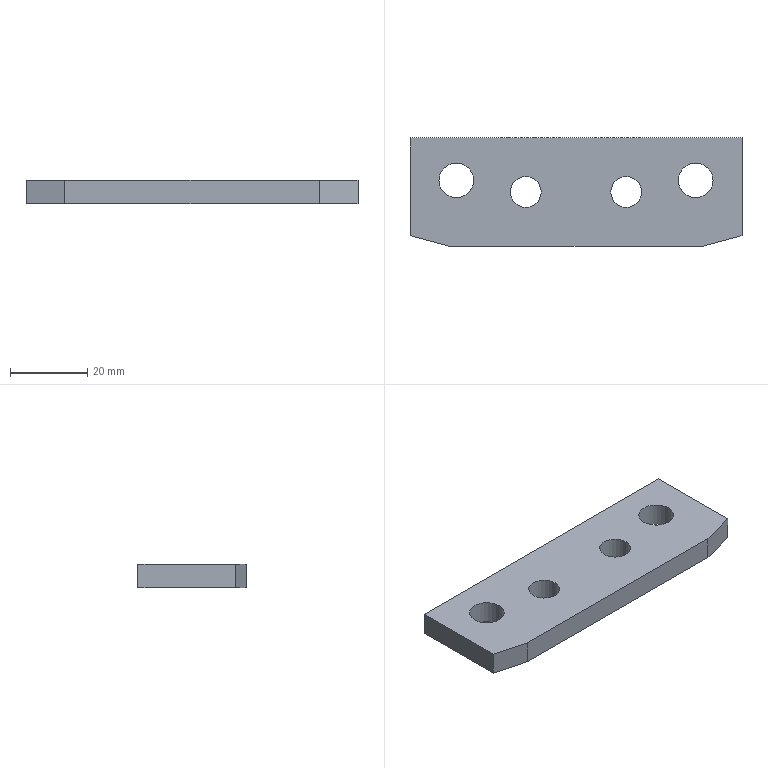Part | STEP file | gslz 2016.10.28-13_id674_x_t | 1 solid | 12 faces | box 86 x 28 x 6 mm | volume 12921 mm3 | plane 8 | cylinder 4 | commonest cylinder face diameters 8 x2 9 x2
STEP:
#1=CARTESIAN_POINT('',(0.,0.,0.));
#2=DIRECTION('',(0.,0.,1.));
#3=DIRECTION('',(1.,0.,0.));
#4=AXIS2_PLACEMENT_3D('',#1,#2,#3);
#5=CARTESIAN_POINT('',(-230.002,281.75,6.));
#6=VERTEX_POINT('',#5);
#7=CARTESIAN_POINT('',(-238.002,281.75,6.));
#8=VERTEX_POINT('',#7);
#9=CARTESIAN_POINT('',(-234.002,281.75,6.));
#10=DIRECTION('',(0.,0.,1.));
#11=DIRECTION('',(-1.,0.,0.));
#12=AXIS2_PLACEMENT_3D('',#9,#10,#11);
#13=CIRCLE('',#12,4.);
#14=CARTESIAN_POINT('',(-234.002,281.75,-73.));
#15=DIRECTION('',(0.,0.,1.));
#16=DIRECTION('',(1.,0.,0.));
#17=AXIS2_PLACEMENT_3D('',#14,#15,#16);
#18=CYLINDRICAL_SURFACE('',#17,4.);
#19=CARTESIAN_POINT('',(-3.142,79.));
#20=DIRECTION('',(1.,0.));
#21=VECTOR('',#20,1.);
#22=LINE('',#19,#21);
#23=(GEOMETRIC_REPRESENTATION_CONTEXT(2)PARAMETRIC_REPRESENTATION_CONTEXT()REPRESENTATION_CONTEXT('',''));
#24=DEFINITIONAL_REPRESENTATION('',(#22),#23);
#25=PCURVE('',#18,#24);
#26=CARTESIAN_POINT('',(-291.002,265.25,6.));
#27=DIRECTION('',(0.,0.,-1.));
#28=DIRECTION('',(-1.,0.,0.));
#29=AXIS2_PLACEMENT_3D('',#26,#27,#28);
#30=PLANE('',#29);
#31=CARTESIAN_POINT('',(-53.,16.5));
#32=CARTESIAN_POINT('',(-53.,9.572));
#33=CARTESIAN_POINT('',(-59.,13.036));
#34=CARTESIAN_POINT('',(-65.,16.5));
#35=CARTESIAN_POINT('',(-59.,19.964));
#36=CARTESIAN_POINT('',(-53.,23.428));
#37=CARTESIAN_POINT('',(-53.,16.5));
#38=(BOUNDED_CURVE()B_SPLINE_CURVE(2,(#31,#32,#33,#34,#35,#36,#37),.UNSPECIFIED.,.T.,.F.)B_SPLINE_CURVE_WITH_KNOTS((1,2,2,2,2,1),(-2.094,0.,2.094,4.189,6.283,8.378),.UNSPECIFIED.)CURVE()GEOMETRIC_REPRESENTATION_ITEM()RATIONAL_B_SPLINE_CURVE((1.,0.5,1.,0.5,1.,0.5,1.))REPRESENTATION_ITEM(''));
#39=(GEOMETRIC_REPRESENTATION_CONTEXT(2)PARAMETRIC_REPRESENTATION_CONTEXT()REPRESENTATION_CONTEXT('',''));
#40=DEFINITIONAL_REPRESENTATION('',(#38),#39);
#41=PCURVE('',#30,#40);
#42=SURFACE_CURVE('',#13,(#25,#41),.PCURVE_S1.);
#43=EDGE_CURVE('',#6,#8,#42,.T.);
#44=ORIENTED_EDGE('',*,*,#43,.F.);
#45=CARTESIAN_POINT('',(-230.002,281.75,0.));
#46=VERTEX_POINT('',#45);
#47=CARTESIAN_POINT('',(-230.002,281.75,0.));
#48=CARTESIAN_POINT('',(-230.002,281.75,6.));
#49=B_SPLINE_CURVE_WITH_KNOTS('',1,(#47,#48),.UNSPECIFIED.,.F.,.F.,(2,2),(73.,79.),.PIECEWISE_BEZIER_KNOTS.);
#50=CARTESIAN_POINT('',(0.,0.));
#51=DIRECTION('',(0.,1.));
#52=VECTOR('',#51,1.);
#53=LINE('',#50,#52);
#54=(GEOMETRIC_REPRESENTATION_CONTEXT(2)PARAMETRIC_REPRESENTATION_CONTEXT()REPRESENTATION_CONTEXT('',''));
#55=DEFINITIONAL_REPRESENTATION('',(#53),#54);
#56=PCURVE('',#18,#55);
#57=CARTESIAN_POINT('',(6.283,0.));
#58=DIRECTION('',(0.,1.));
#59=VECTOR('',#58,1.);
#60=LINE('',#57,#59);
#61=(GEOMETRIC_REPRESENTATION_CONTEXT(2)PARAMETRIC_REPRESENTATION_CONTEXT()REPRESENTATION_CONTEXT('',''));
#62=DEFINITIONAL_REPRESENTATION('',(#60),#61);
#63=PCURVE('',#18,#62);
#64=SEAM_CURVE('',#49,(#56,#63),.PCURVE_S1.);
#65=EDGE_CURVE('',#46,#6,#64,.T.);
#66=ORIENTED_EDGE('',*,*,#65,.F.);
#67=CARTESIAN_POINT('',(-234.002,281.75,0.));
#68=DIRECTION('',(0.,0.,-1.));
#69=DIRECTION('',(1.,0.,0.));
#70=AXIS2_PLACEMENT_3D('',#67,#68,#69);
#71=CIRCLE('',#70,4.);
#72=CARTESIAN_POINT('',(6.283,73.));
#73=DIRECTION('',(-1.,0.));
#74=VECTOR('',#73,1.);
#75=LINE('',#72,#74);
#76=(GEOMETRIC_REPRESENTATION_CONTEXT(2)PARAMETRIC_REPRESENTATION_CONTEXT()REPRESENTATION_CONTEXT('',''));
#77=DEFINITIONAL_REPRESENTATION('',(#75),#76);
#78=PCURVE('',#18,#77);
#79=CARTESIAN_POINT('',(-331.002,295.75,0.));
#80=DIRECTION('',(0.,0.,1.));
#81=DIRECTION('',(1.,0.,0.));
#82=AXIS2_PLACEMENT_3D('',#79,#80,#81);
#83=PLANE('',#82);
#84=CARTESIAN_POINT('',(101.,-14.));
#85=CARTESIAN_POINT('',(101.,-20.928));
#86=CARTESIAN_POINT('',(95.,-17.464));
#87=CARTESIAN_POINT('',(89.,-14.));
#88=CARTESIAN_POINT('',(95.,-10.536));
#89=CARTESIAN_POINT('',(101.,-7.072));
#90=CARTESIAN_POINT('',(101.,-14.));
#91=(BOUNDED_CURVE()B_SPLINE_CURVE(2,(#84,#85,#86,#87,#88,#89,#90),.UNSPECIFIED.,.T.,.F.)B_SPLINE_CURVE_WITH_KNOTS((1,2,2,2,2,1),(-2.094,0.,2.094,4.189,6.283,8.378),.UNSPECIFIED.)CURVE()GEOMETRIC_REPRESENTATION_ITEM()RATIONAL_B_SPLINE_CURVE((1.,0.5,1.,0.5,1.,0.5,1.))REPRESENTATION_ITEM(''));
#92=(GEOMETRIC_REPRESENTATION_CONTEXT(2)PARAMETRIC_REPRESENTATION_CONTEXT()REPRESENTATION_CONTEXT('',''));
#93=DEFINITIONAL_REPRESENTATION('',(#91),#92);
#94=PCURVE('',#83,#93);
#95=SURFACE_CURVE('',#71,(#78,#94),.PCURVE_S1.);
#96=EDGE_CURVE('',#46,#46,#95,.T.);
#97=ORIENTED_EDGE('',*,*,#96,.F.);
#98=ORIENTED_EDGE('',*,*,#65,.T.);
#99=CARTESIAN_POINT('',(-234.002,281.75,6.));
#100=DIRECTION('',(0.,0.,1.));
#101=DIRECTION('',(-1.,0.,0.));
#102=AXIS2_PLACEMENT_3D('',#99,#100,#101);
#103=CIRCLE('',#102,4.);
#104=CARTESIAN_POINT('',(3.142,79.));
#105=DIRECTION('',(1.,0.));
#106=VECTOR('',#105,1.);
#107=LINE('',#104,#106);
#108=(GEOMETRIC_REPRESENTATION_CONTEXT(2)PARAMETRIC_REPRESENTATION_CONTEXT()REPRESENTATION_CONTEXT('',''));
#109=DEFINITIONAL_REPRESENTATION('',(#107),#108);
#110=PCURVE('',#18,#109);
#111=CARTESIAN_POINT('',(-53.,16.5));
#112=CARTESIAN_POINT('',(-53.,9.572));
#113=CARTESIAN_POINT('',(-59.,13.036));
#114=CARTESIAN_POINT('',(-65.,16.5));
#115=CARTESIAN_POINT('',(-59.,19.964));
#116=CARTESIAN_POINT('',(-53.,23.428));
#117=CARTESIAN_POINT('',(-53.,16.5));
#118=(BOUNDED_CURVE()B_SPLINE_CURVE(2,(#111,#112,#113,#114,#115,#116,#117),.UNSPECIFIED.,.T.,.F.)B_SPLINE_CURVE_WITH_KNOTS((1,2,2,2,2,1),(-2.094,0.,2.094,4.189,6.283,8.378),.UNSPECIFIED.)CURVE()GEOMETRIC_REPRESENTATION_ITEM()RATIONAL_B_SPLINE_CURVE((1.,0.5,1.,0.5,1.,0.5,1.))REPRESENTATION_ITEM(''));
#119=(GEOMETRIC_REPRESENTATION_CONTEXT(2)PARAMETRIC_REPRESENTATION_CONTEXT()REPRESENTATION_CONTEXT('',''));
#120=DEFINITIONAL_REPRESENTATION('',(#118),#119);
#121=PCURVE('',#30,#120);
#122=SURFACE_CURVE('',#103,(#110,#121),.PCURVE_S1.);
#123=EDGE_CURVE('',#8,#6,#122,.T.);
#124=ORIENTED_EDGE('',*,*,#123,.F.);
#125=EDGE_LOOP('',(#44,#66,#97,#98,#124));
#126=FACE_BOUND('',#125,.F.);
#127=ADVANCED_FACE('',(#126),#18,.F.);
#128=CARTESIAN_POINT('',(-212.002,281.75,6.));
#129=VERTEX_POINT('',#128);
#130=CARTESIAN_POINT('',(-204.002,281.75,6.));
#131=VERTEX_POINT('',#130);
#132=CARTESIAN_POINT('',(-208.002,281.75,6.));
#133=DIRECTION('',(0.,0.,-1.));
#134=DIRECTION('',(-1.,0.,0.));
#135=AXIS2_PLACEMENT_3D('',#132,#133,#134);
#136=CIRCLE('',#135,4.);
#137=CARTESIAN_POINT('',(-208.002,281.75,-73.));
#138=DIRECTION('',(0.,0.,1.));
#139=DIRECTION('',(1.,0.,0.));
#140=AXIS2_PLACEMENT_3D('',#137,#138,#139);
#141=CYLINDRICAL_SURFACE('',#140,4.);
#142=CARTESIAN_POINT('',(3.142,79.));
#143=DIRECTION('',(-1.,0.));
#144=VECTOR('',#143,1.);
#145=LINE('',#142,#144);
#146=(GEOMETRIC_REPRESENTATION_CONTEXT(2)PARAMETRIC_REPRESENTATION_CONTEXT()REPRESENTATION_CONTEXT('',''));
#147=DEFINITIONAL_REPRESENTATION('',(#145),#146);
#148=PCURVE('',#141,#147);
#149=CARTESIAN_POINT('',(-83.,16.5));
#150=DIRECTION('',(1.,0.));
#151=AXIS2_PLACEMENT_2D('',#149,#150);
#152=CIRCLE('',#151,4.);
#153=(GEOMETRIC_REPRESENTATION_CONTEXT(2)PARAMETRIC_REPRESENTATION_CONTEXT()REPRESENTATION_CONTEXT('',''));
#154=DEFINITIONAL_REPRESENTATION('',(#152),#153);
#155=PCURVE('',#30,#154);
#156=SURFACE_CURVE('',#136,(#148,#155),.PCURVE_S1.);
#157=EDGE_CURVE('',#129,#131,#156,.T.);
#158=ORIENTED_EDGE('',*,*,#157,.T.);
#159=CARTESIAN_POINT('',(-204.002,281.75,0.));
#160=VERTEX_POINT('',#159);
#161=CARTESIAN_POINT('',(-204.002,281.75,0.));
#162=CARTESIAN_POINT('',(-204.002,281.75,6.));
#163=B_SPLINE_CURVE_WITH_KNOTS('',1,(#161,#162),.UNSPECIFIED.,.F.,.F.,(2,2),(73.,79.),.PIECEWISE_BEZIER_KNOTS.);
#164=CARTESIAN_POINT('',(0.,0.));
#165=DIRECTION('',(0.,1.));
#166=VECTOR('',#165,1.);
#167=LINE('',#164,#166);
#168=(GEOMETRIC_REPRESENTATION_CONTEXT(2)PARAMETRIC_REPRESENTATION_CONTEXT()REPRESENTATION_CONTEXT('',''));
#169=DEFINITIONAL_REPRESENTATION('',(#167),#168);
#170=PCURVE('',#141,#169);
#171=CARTESIAN_POINT('',(6.283,0.));
#172=DIRECTION('',(0.,1.));
#173=VECTOR('',#172,1.);
#174=LINE('',#171,#173);
#175=(GEOMETRIC_REPRESENTATION_CONTEXT(2)PARAMETRIC_REPRESENTATION_CONTEXT()REPRESENTATION_CONTEXT('',''));
#176=DEFINITIONAL_REPRESENTATION('',(#174),#175);
#177=PCURVE('',#141,#176);
#178=SEAM_CURVE('',#163,(#170,#177),.PCURVE_S1.);
#179=EDGE_CURVE('',#160,#131,#178,.T.);
#180=ORIENTED_EDGE('',*,*,#179,.F.);
#181=CARTESIAN_POINT('',(-208.002,281.75,0.));
#182=DIRECTION('',(0.,0.,1.));
#183=DIRECTION('',(1.,0.,0.));
#184=AXIS2_PLACEMENT_3D('',#181,#182,#183);
#185=CIRCLE('',#184,4.);
#186=CARTESIAN_POINT('',(0.,73.));
#187=DIRECTION('',(1.,0.));
#188=VECTOR('',#187,1.);
#189=LINE('',#186,#188);
#190=(GEOMETRIC_REPRESENTATION_CONTEXT(2)PARAMETRIC_REPRESENTATION_CONTEXT()REPRESENTATION_CONTEXT('',''));
#191=DEFINITIONAL_REPRESENTATION('',(#189),#190);
#192=PCURVE('',#141,#191);
#193=CARTESIAN_POINT('',(123.,-14.));
#194=DIRECTION('',(1.,0.));
#195=AXIS2_PLACEMENT_2D('',#193,#194);
#196=CIRCLE('',#195,4.);
#197=(GEOMETRIC_REPRESENTATION_CONTEXT(2)PARAMETRIC_REPRESENTATION_CONTEXT()REPRESENTATION_CONTEXT('',''));
#198=DEFINITIONAL_REPRESENTATION('',(#196),#197);
#199=PCURVE('',#83,#198);
#200=SURFACE_CURVE('',#185,(#192,#199),.PCURVE_S1.);
#201=EDGE_CURVE('',#160,#160,#200,.T.);
#202=ORIENTED_EDGE('',*,*,#201,.T.);
#203=ORIENTED_EDGE('',*,*,#179,.T.);
#204=CARTESIAN_POINT('',(-208.002,281.75,6.));
#205=DIRECTION('',(0.,0.,-1.));
#206=DIRECTION('',(-1.,0.,0.));
#207=AXIS2_PLACEMENT_3D('',#204,#205,#206);
#208=CIRCLE('',#207,4.);
#209=CARTESIAN_POINT('',(9.425,79.));
#210=DIRECTION('',(-1.,0.));
#211=VECTOR('',#210,1.);
#212=LINE('',#209,#211);
#213=(GEOMETRIC_REPRESENTATION_CONTEXT(2)PARAMETRIC_REPRESENTATION_CONTEXT()REPRESENTATION_CONTEXT('',''));
#214=DEFINITIONAL_REPRESENTATION('',(#212),#213);
#215=PCURVE('',#141,#214);
#216=CARTESIAN_POINT('',(-83.,16.5));
#217=DIRECTION('',(1.,0.));
#218=AXIS2_PLACEMENT_2D('',#216,#217);
#219=CIRCLE('',#218,4.);
#220=(GEOMETRIC_REPRESENTATION_CONTEXT(2)PARAMETRIC_REPRESENTATION_CONTEXT()REPRESENTATION_CONTEXT('',''));
#221=DEFINITIONAL_REPRESENTATION('',(#219),#220);
#222=PCURVE('',#30,#221);
#223=SURFACE_CURVE('',#208,(#215,#222),.PCURVE_S1.);
#224=EDGE_CURVE('',#131,#129,#223,.T.);
#225=ORIENTED_EDGE('',*,*,#224,.T.);
#226=EDGE_LOOP('',(#158,#180,#202,#203,#225));
#227=FACE_BOUND('',#226,.F.);
#228=ADVANCED_FACE('',(#227),#141,.F.);
#229=CARTESIAN_POINT('',(-256.502,284.75,6.));
#230=VERTEX_POINT('',#229);
#231=CARTESIAN_POINT('',(-252.002,284.75,6.));
#232=DIRECTION('',(0.,0.,-1.));
#233=DIRECTION('',(-1.,0.,0.));
#234=AXIS2_PLACEMENT_3D('',#231,#232,#233);
#235=CIRCLE('',#234,4.5);
#236=CARTESIAN_POINT('',(-252.002,284.75,47.));
#237=DIRECTION('',(0.,0.,-1.));
#238=DIRECTION('',(-1.,0.,0.));
#239=AXIS2_PLACEMENT_3D('',#236,#237,#238);
#240=CYLINDRICAL_SURFACE('',#239,4.5);
#241=CARTESIAN_POINT('',(0.,41.));
#242=DIRECTION('',(1.,0.));
#243=VECTOR('',#242,1.);
#244=LINE('',#241,#243);
#245=(GEOMETRIC_REPRESENTATION_CONTEXT(2)PARAMETRIC_REPRESENTATION_CONTEXT()REPRESENTATION_CONTEXT('',''));
#246=DEFINITIONAL_REPRESENTATION('',(#244),#245);
#247=PCURVE('',#240,#246);
#248=CARTESIAN_POINT('',(-39.,19.5));
#249=DIRECTION('',(1.,0.));
#250=AXIS2_PLACEMENT_2D('',#248,#249);
#251=CIRCLE('',#250,4.5);
#252=(GEOMETRIC_REPRESENTATION_CONTEXT(2)PARAMETRIC_REPRESENTATION_CONTEXT()REPRESENTATION_CONTEXT('',''));
#253=DEFINITIONAL_REPRESENTATION('',(#251),#252);
#254=PCURVE('',#30,#253);
#255=SURFACE_CURVE('',#235,(#247,#254),.PCURVE_S1.);
#256=EDGE_CURVE('',#230,#230,#255,.T.);
#257=ORIENTED_EDGE('',*,*,#256,.T.);
#258=CARTESIAN_POINT('',(-256.502,284.75,0.));
#259=VERTEX_POINT('',#258);
#260=CARTESIAN_POINT('',(-256.502,284.75,6.));
#261=CARTESIAN_POINT('',(-256.502,284.75,0.));
#262=B_SPLINE_CURVE_WITH_KNOTS('',1,(#260,#261),.UNSPECIFIED.,.F.,.F.,(2,2),(41.,47.),.PIECEWISE_BEZIER_KNOTS.);
#263=CARTESIAN_POINT('',(6.283,0.));
#264=DIRECTION('',(0.,1.));
#265=VECTOR('',#264,1.);
#266=LINE('',#263,#265);
#267=(GEOMETRIC_REPRESENTATION_CONTEXT(2)PARAMETRIC_REPRESENTATION_CONTEXT()REPRESENTATION_CONTEXT('',''));
#268=DEFINITIONAL_REPRESENTATION('',(#266),#267);
#269=PCURVE('',#240,#268);
#270=CARTESIAN_POINT('',(0.,0.));
#271=DIRECTION('',(0.,1.));
#272=VECTOR('',#271,1.);
#273=LINE('',#270,#272);
#274=(GEOMETRIC_REPRESENTATION_CONTEXT(2)PARAMETRIC_REPRESENTATION_CONTEXT()REPRESENTATION_CONTEXT('',''));
#275=DEFINITIONAL_REPRESENTATION('',(#273),#274);
#276=PCURVE('',#240,#275);
#277=SEAM_CURVE('',#262,(#269,#276),.PCURVE_S1.);
#278=EDGE_CURVE('',#230,#259,#277,.T.);
#279=ORIENTED_EDGE('',*,*,#278,.T.);
#280=CARTESIAN_POINT('',(-247.502,284.75,0.));
#281=VERTEX_POINT('',#280);
#282=CARTESIAN_POINT('',(-252.002,284.75,0.));
#283=DIRECTION('',(0.,0.,1.));
#284=DIRECTION('',(1.,0.,0.));
#285=AXIS2_PLACEMENT_3D('',#282,#283,#284);
#286=CIRCLE('',#285,4.5);
#287=CARTESIAN_POINT('',(9.425,47.));
#288=DIRECTION('',(-1.,0.));
#289=VECTOR('',#288,1.);
#290=LINE('',#287,#289);
#291=(GEOMETRIC_REPRESENTATION_CONTEXT(2)PARAMETRIC_REPRESENTATION_CONTEXT()REPRESENTATION_CONTEXT('',''));
#292=DEFINITIONAL_REPRESENTATION('',(#290),#291);
#293=PCURVE('',#240,#292);
#294=CARTESIAN_POINT('',(79.,-11.));
#295=DIRECTION('',(1.,0.));
#296=AXIS2_PLACEMENT_2D('',#294,#295);
#297=CIRCLE('',#296,4.5);
#298=(GEOMETRIC_REPRESENTATION_CONTEXT(2)PARAMETRIC_REPRESENTATION_CONTEXT()REPRESENTATION_CONTEXT('',''));
#299=DEFINITIONAL_REPRESENTATION('',(#297),#298);
#300=PCURVE('',#83,#299);
#301=SURFACE_CURVE('',#286,(#293,#300),.PCURVE_S1.);
#302=EDGE_CURVE('',#259,#281,#301,.T.);
#303=ORIENTED_EDGE('',*,*,#302,.T.);
#304=CARTESIAN_POINT('',(-252.002,284.75,0.));
#305=DIRECTION('',(0.,0.,1.));
#306=DIRECTION('',(1.,0.,0.));
#307=AXIS2_PLACEMENT_3D('',#304,#305,#306);
#308=CIRCLE('',#307,4.5);
#309=CARTESIAN_POINT('',(3.142,47.));
#310=DIRECTION('',(-1.,0.));
#311=VECTOR('',#310,1.);
#312=LINE('',#309,#311);
#313=(GEOMETRIC_REPRESENTATION_CONTEXT(2)PARAMETRIC_REPRESENTATION_CONTEXT()REPRESENTATION_CONTEXT('',''));
#314=DEFINITIONAL_REPRESENTATION('',(#312),#313);
#315=PCURVE('',#240,#314);
#316=CARTESIAN_POINT('',(79.,-11.));
#317=DIRECTION('',(1.,0.));
#318=AXIS2_PLACEMENT_2D('',#316,#317);
#319=CIRCLE('',#318,4.5);
#320=(GEOMETRIC_REPRESENTATION_CONTEXT(2)PARAMETRIC_REPRESENTATION_CONTEXT()REPRESENTATION_CONTEXT('',''));
#321=DEFINITIONAL_REPRESENTATION('',(#319),#320);
#322=PCURVE('',#83,#321);
#323=SURFACE_CURVE('',#308,(#315,#322),.PCURVE_S1.);
#324=EDGE_CURVE('',#281,#259,#323,.T.);
#325=ORIENTED_EDGE('',*,*,#324,.T.);
#326=ORIENTED_EDGE('',*,*,#278,.F.);
#327=EDGE_LOOP('',(#257,#279,#303,#325,#326));
#328=FACE_BOUND('',#327,.F.);
#329=ADVANCED_FACE('',(#328),#240,.F.);
#330=CARTESIAN_POINT('',(-188.001,267.75,0.));
#331=VERTEX_POINT('',#330);
#332=CARTESIAN_POINT('',(-188.001,267.75,6.));
#333=VERTEX_POINT('',#332);
#334=CARTESIAN_POINT('',(-188.001,267.75,8.));
#335=DIRECTION('',(0.,0.,1.));
#336=VECTOR('',#335,1.);
#337=LINE('',#334,#336);
#338=CARTESIAN_POINT('',(-321.,267.75,8.));
#339=DIRECTION('',(0.,1.,0.));
#340=DIRECTION('',(0.,0.,1.));
#341=AXIS2_PLACEMENT_3D('',#338,#339,#340);
#342=PLANE('',#341);
#343=CARTESIAN_POINT('',(0.,132.999));
#344=DIRECTION('',(1.,0.));
#345=VECTOR('',#344,1.);
#346=LINE('',#343,#345);
#347=(GEOMETRIC_REPRESENTATION_CONTEXT(2)PARAMETRIC_REPRESENTATION_CONTEXT()REPRESENTATION_CONTEXT('',''));
#348=DEFINITIONAL_REPRESENTATION('',(#346),#347);
#349=PCURVE('',#342,#348);
#350=CARTESIAN_POINT('',(-188.001,267.75,8.));
#351=DIRECTION('',(-0.2588,0.9659,0.));
#352=DIRECTION('',(-0.9659,-0.2588,0.));
#353=AXIS2_PLACEMENT_3D('',#350,#351,#352);
#354=PLANE('',#353);
#355=CARTESIAN_POINT('',(0.,0.));
#356=DIRECTION('',(0.,1.));
#357=VECTOR('',#356,1.);
#358=LINE('',#355,#357);
#359=(GEOMETRIC_REPRESENTATION_CONTEXT(2)PARAMETRIC_REPRESENTATION_CONTEXT()REPRESENTATION_CONTEXT('',''));
#360=DEFINITIONAL_REPRESENTATION('',(#358),#359);
#361=PCURVE('',#354,#360);
#362=SURFACE_CURVE('',#337,(#349,#361),.PCURVE_S1.);
#363=EDGE_CURVE('',#331,#333,#362,.T.);
#364=ORIENTED_EDGE('',*,*,#363,.T.);
#365=CARTESIAN_POINT('',(-254.,267.75,6.));
#366=VERTEX_POINT('',#365);
#367=CARTESIAN_POINT('',(-321.,267.75,6.));
#368=DIRECTION('',(-1.,0.,0.));
#369=VECTOR('',#368,1.);
#370=LINE('',#367,#369);
#371=CARTESIAN_POINT('',(-2.,0.));
#372=DIRECTION('',(0.,-1.));
#373=VECTOR('',#372,1.);
#374=LINE('',#371,#373);
#375=(GEOMETRIC_REPRESENTATION_CONTEXT(2)PARAMETRIC_REPRESENTATION_CONTEXT()REPRESENTATION_CONTEXT('',''));
#376=DEFINITIONAL_REPRESENTATION('',(#374),#375);
#377=PCURVE('',#342,#376);
#378=CARTESIAN_POINT('',(29.998,2.5));
#379=DIRECTION('',(1.,0.));
#380=VECTOR('',#379,1.);
#381=LINE('',#378,#380);
#382=(GEOMETRIC_REPRESENTATION_CONTEXT(2)PARAMETRIC_REPRESENTATION_CONTEXT()REPRESENTATION_CONTEXT('',''));
#383=DEFINITIONAL_REPRESENTATION('',(#381),#382);
#384=PCURVE('',#30,#383);
#385=SURFACE_CURVE('',#370,(#377,#384),.PCURVE_S1.);
#386=EDGE_CURVE('',#333,#366,#385,.T.);
#387=ORIENTED_EDGE('',*,*,#386,.T.);
#388=CARTESIAN_POINT('',(-254.,267.75,0.));
#389=VERTEX_POINT('',#388);
#390=CARTESIAN_POINT('',(-254.,267.75,8.));
#391=DIRECTION('',(0.,0.,1.));
#392=VECTOR('',#391,1.);
#393=LINE('',#390,#392);
#394=CARTESIAN_POINT('',(0.,67.));
#395=DIRECTION('',(1.,0.));
#396=VECTOR('',#395,1.);
#397=LINE('',#394,#396);
#398=(GEOMETRIC_REPRESENTATION_CONTEXT(2)PARAMETRIC_REPRESENTATION_CONTEXT()REPRESENTATION_CONTEXT('',''));
#399=DEFINITIONAL_REPRESENTATION('',(#397),#398);
#400=PCURVE('',#342,#399);
#401=CARTESIAN_POINT('',(-264.002,270.43,8.));
#402=DIRECTION('',(0.2588,0.9659,0.));
#403=DIRECTION('',(-0.9659,0.2588,0.));
#404=AXIS2_PLACEMENT_3D('',#401,#402,#403);
#405=PLANE('',#404);
#406=CARTESIAN_POINT('',(-10.355,0.));
#407=DIRECTION('',(0.,1.));
#408=VECTOR('',#407,1.);
#409=LINE('',#406,#408);
#410=(GEOMETRIC_REPRESENTATION_CONTEXT(2)PARAMETRIC_REPRESENTATION_CONTEXT()REPRESENTATION_CONTEXT('',''));
#411=DEFINITIONAL_REPRESENTATION('',(#409),#410);
#412=PCURVE('',#405,#411);
#413=SURFACE_CURVE('',#393,(#400,#412),.PCURVE_S1.);
#414=EDGE_CURVE('',#389,#366,#413,.T.);
#415=ORIENTED_EDGE('',*,*,#414,.F.);
#416=CARTESIAN_POINT('',(-321.,267.75,0.));
#417=DIRECTION('',(1.,0.,0.));
#418=VECTOR('',#417,1.);
#419=LINE('',#416,#418);
#420=CARTESIAN_POINT('',(-8.,0.));
#421=DIRECTION('',(0.,1.));
#422=VECTOR('',#421,1.);
#423=LINE('',#420,#422);
#424=(GEOMETRIC_REPRESENTATION_CONTEXT(2)PARAMETRIC_REPRESENTATION_CONTEXT()REPRESENTATION_CONTEXT('',''));
#425=DEFINITIONAL_REPRESENTATION('',(#423),#424);
#426=PCURVE('',#342,#425);
#427=CARTESIAN_POINT('',(10.002,-28.));
#428=DIRECTION('',(1.,0.));
#429=VECTOR('',#428,1.);
#430=LINE('',#427,#429);
#431=(GEOMETRIC_REPRESENTATION_CONTEXT(2)PARAMETRIC_REPRESENTATION_CONTEXT()REPRESENTATION_CONTEXT('',''));
#432=DEFINITIONAL_REPRESENTATION('',(#430),#431);
#433=PCURVE('',#83,#432);
#434=SURFACE_CURVE('',#419,(#426,#433),.PCURVE_S1.);
#435=EDGE_CURVE('',#389,#331,#434,.T.);
#436=ORIENTED_EDGE('',*,*,#435,.T.);
#437=EDGE_LOOP('',(#364,#387,#415,#436));
#438=FACE_BOUND('',#437,.T.);
#439=ADVANCED_FACE('',(#438),#342,.F.);
#440=CARTESIAN_POINT('',(-178.002,270.429,6.));
#441=VERTEX_POINT('',#440);
#442=CARTESIAN_POINT('',(-178.002,270.429,0.));
#443=VERTEX_POINT('',#442);
#444=CARTESIAN_POINT('',(-178.002,270.429,8.));
#445=DIRECTION('',(0.,0.,-1.));
#446=VECTOR('',#445,1.);
#447=LINE('',#444,#446);
#448=CARTESIAN_POINT('',(-10.352,0.));
#449=DIRECTION('',(0.,-1.));
#450=VECTOR('',#449,1.);
#451=LINE('',#448,#450);
#452=(GEOMETRIC_REPRESENTATION_CONTEXT(2)PARAMETRIC_REPRESENTATION_CONTEXT()REPRESENTATION_CONTEXT('',''));
#453=DEFINITIONAL_REPRESENTATION('',(#451),#452);
#454=PCURVE('',#354,#453);
#455=CARTESIAN_POINT('',(-178.002,262.75,16.));
#456=DIRECTION('',(-1.,0.,0.));
#457=DIRECTION('',(0.,0.,1.));
#458=AXIS2_PLACEMENT_3D('',#455,#456,#457);
#459=PLANE('',#458);
#460=CARTESIAN_POINT('',(-8.,7.679));
#461=DIRECTION('',(-1.,0.));
#462=VECTOR('',#461,1.);
#463=LINE('',#460,#462);
#464=(GEOMETRIC_REPRESENTATION_CONTEXT(2)PARAMETRIC_REPRESENTATION_CONTEXT()REPRESENTATION_CONTEXT('',''));
#465=DEFINITIONAL_REPRESENTATION('',(#463),#464);
#466=PCURVE('',#459,#465);
#467=SURFACE_CURVE('',#447,(#454,#466),.PCURVE_S1.);
#468=EDGE_CURVE('',#441,#443,#467,.T.);
#469=ORIENTED_EDGE('',*,*,#468,.F.);
#470=CARTESIAN_POINT('',(-188.001,267.75,6.));
#471=DIRECTION('',(-0.9659,-0.2588,0.));
#472=VECTOR('',#471,1.);
#473=LINE('',#470,#472);
#474=CARTESIAN_POINT('',(0.,-2.));
#475=DIRECTION('',(1.,0.));
#476=VECTOR('',#475,1.);
#477=LINE('',#474,#476);
#478=(GEOMETRIC_REPRESENTATION_CONTEXT(2)PARAMETRIC_REPRESENTATION_CONTEXT()REPRESENTATION_CONTEXT('',''));
#479=DEFINITIONAL_REPRESENTATION('',(#477),#478);
#480=PCURVE('',#354,#479);
#481=CARTESIAN_POINT('',(-103.001,2.5));
#482=DIRECTION('',(0.9659,-0.2588));
#483=VECTOR('',#482,1.);
#484=LINE('',#481,#483);
#485=(GEOMETRIC_REPRESENTATION_CONTEXT(2)PARAMETRIC_REPRESENTATION_CONTEXT()REPRESENTATION_CONTEXT('',''));
#486=DEFINITIONAL_REPRESENTATION('',(#484),#485);
#487=PCURVE('',#30,#486);
#488=SURFACE_CURVE('',#473,(#480,#487),.PCURVE_S1.);
#489=EDGE_CURVE('',#441,#333,#488,.T.);
#490=ORIENTED_EDGE('',*,*,#489,.T.);
#491=ORIENTED_EDGE('',*,*,#363,.F.);
#492=CARTESIAN_POINT('',(-188.001,267.75,0.));
#493=DIRECTION('',(0.9659,0.2588,0.));
#494=VECTOR('',#493,1.);
#495=LINE('',#492,#494);
#496=CARTESIAN_POINT('',(0.,-8.));
#497=DIRECTION('',(-1.,0.));
#498=VECTOR('',#497,1.);
#499=LINE('',#496,#498);
#500=(GEOMETRIC_REPRESENTATION_CONTEXT(2)PARAMETRIC_REPRESENTATION_CONTEXT()REPRESENTATION_CONTEXT('',''));
#501=DEFINITIONAL_REPRESENTATION('',(#499),#500);
#502=PCURVE('',#354,#501);
#503=CARTESIAN_POINT('',(143.001,-28.));
#504=DIRECTION('',(0.9659,0.2588));
#505=VECTOR('',#504,1.);
#506=LINE('',#503,#505);
#507=(GEOMETRIC_REPRESENTATION_CONTEXT(2)PARAMETRIC_REPRESENTATION_CONTEXT()REPRESENTATION_CONTEXT('',''));
#508=DEFINITIONAL_REPRESENTATION('',(#506),#507);
#509=PCURVE('',#83,#508);
#510=SURFACE_CURVE('',#495,(#502,#509),.PCURVE_S1.);
#511=EDGE_CURVE('',#331,#443,#510,.T.);
#512=ORIENTED_EDGE('',*,*,#511,.T.);
#513=EDGE_LOOP('',(#469,#490,#491,#512));
#514=FACE_BOUND('',#513,.T.);
#515=ADVANCED_FACE('',(#514),#354,.F.);
#516=CARTESIAN_POINT('',(-178.002,295.75,6.));
#517=VERTEX_POINT('',#516);
#518=CARTESIAN_POINT('',(-178.002,295.75,0.));
#519=VERTEX_POINT('',#518);
#520=CARTESIAN_POINT('',(-178.002,295.75,16.));
#521=DIRECTION('',(0.,0.,-1.));
#522=VECTOR('',#521,1.);
#523=LINE('',#520,#522);
#524=CARTESIAN_POINT('',(0.,33.));
#525=DIRECTION('',(-1.,0.));
#526=VECTOR('',#525,1.);
#527=LINE('',#524,#526);
#528=(GEOMETRIC_REPRESENTATION_CONTEXT(2)PARAMETRIC_REPRESENTATION_CONTEXT()REPRESENTATION_CONTEXT('',''));
#529=DEFINITIONAL_REPRESENTATION('',(#527),#528);
#530=PCURVE('',#459,#529);
#531=CARTESIAN_POINT('',(-251.002,295.75,16.));
#532=DIRECTION('',(0.,-1.,0.));
#533=DIRECTION('',(0.,0.,-1.));
#534=AXIS2_PLACEMENT_3D('',#531,#532,#533);
#535=PLANE('',#534);
#536=CARTESIAN_POINT('',(0.,73.));
#537=DIRECTION('',(1.,0.));
#538=VECTOR('',#537,1.);
#539=LINE('',#536,#538);
#540=(GEOMETRIC_REPRESENTATION_CONTEXT(2)PARAMETRIC_REPRESENTATION_CONTEXT()REPRESENTATION_CONTEXT('',''));
#541=DEFINITIONAL_REPRESENTATION('',(#539),#540);
#542=PCURVE('',#535,#541);
#543=SURFACE_CURVE('',#523,(#530,#542),.PCURVE_S1.);
#544=EDGE_CURVE('',#517,#519,#543,.T.);
#545=ORIENTED_EDGE('',*,*,#544,.F.);
#546=CARTESIAN_POINT('',(-178.002,262.75,6.));
#547=DIRECTION('',(0.,-1.,0.));
#548=VECTOR('',#547,1.);
#549=LINE('',#546,#548);
#550=CARTESIAN_POINT('',(-10.,0.));
#551=DIRECTION('',(0.,-1.));
#552=VECTOR('',#551,1.);
#553=LINE('',#550,#552);
#554=(GEOMETRIC_REPRESENTATION_CONTEXT(2)PARAMETRIC_REPRESENTATION_CONTEXT()REPRESENTATION_CONTEXT('',''));
#555=DEFINITIONAL_REPRESENTATION('',(#553),#554);
#556=PCURVE('',#459,#555);
#557=CARTESIAN_POINT('',(-113.,-2.5));
#558=DIRECTION('',(0.,-1.));
#559=VECTOR('',#558,1.);
#560=LINE('',#557,#559);
#561=(GEOMETRIC_REPRESENTATION_CONTEXT(2)PARAMETRIC_REPRESENTATION_CONTEXT()REPRESENTATION_CONTEXT('',''));
#562=DEFINITIONAL_REPRESENTATION('',(#560),#561);
#563=PCURVE('',#30,#562);
#564=SURFACE_CURVE('',#549,(#556,#563),.PCURVE_S1.);
#565=EDGE_CURVE('',#517,#441,#564,.T.);
#566=ORIENTED_EDGE('',*,*,#565,.T.);
#567=ORIENTED_EDGE('',*,*,#468,.T.);
#568=CARTESIAN_POINT('',(-178.002,262.75,0.));
#569=DIRECTION('',(0.,1.,0.));
#570=VECTOR('',#569,1.);
#571=LINE('',#568,#570);
#572=CARTESIAN_POINT('',(-16.,0.));
#573=DIRECTION('',(0.,1.));
#574=VECTOR('',#573,1.);
#575=LINE('',#572,#574);
#576=(GEOMETRIC_REPRESENTATION_CONTEXT(2)PARAMETRIC_REPRESENTATION_CONTEXT()REPRESENTATION_CONTEXT('',''));
#577=DEFINITIONAL_REPRESENTATION('',(#575),#576);
#578=PCURVE('',#459,#577);
#579=CARTESIAN_POINT('',(153.,-33.));
#580=DIRECTION('',(0.,1.));
#581=VECTOR('',#580,1.);
#582=LINE('',#579,#581);
#583=(GEOMETRIC_REPRESENTATION_CONTEXT(2)PARAMETRIC_REPRESENTATION_CONTEXT()REPRESENTATION_CONTEXT('',''));
#584=DEFINITIONAL_REPRESENTATION('',(#582),#583);
#585=PCURVE('',#83,#584);
#586=SURFACE_CURVE('',#571,(#578,#585),.PCURVE_S1.);
#587=EDGE_CURVE('',#443,#519,#586,.T.);
#588=ORIENTED_EDGE('',*,*,#587,.T.);
#589=EDGE_LOOP('',(#545,#566,#567,#588));
#590=FACE_BOUND('',#589,.T.);
#591=ADVANCED_FACE('',(#590),#459,.F.);
#592=CARTESIAN_POINT('',(-264.002,295.75,6.));
#593=VERTEX_POINT('',#592);
#594=CARTESIAN_POINT('',(-264.002,295.75,0.));
#595=VERTEX_POINT('',#594);
#596=CARTESIAN_POINT('',(-264.002,295.75,16.));
#597=DIRECTION('',(0.,0.,-1.));
#598=VECTOR('',#597,1.);
#599=LINE('',#596,#598);
#600=CARTESIAN_POINT('',(0.,-13.));
#601=DIRECTION('',(1.,0.));
#602=VECTOR('',#601,1.);
#603=LINE('',#600,#602);
#604=(GEOMETRIC_REPRESENTATION_CONTEXT(2)PARAMETRIC_REPRESENTATION_CONTEXT()REPRESENTATION_CONTEXT('',''));
#605=DEFINITIONAL_REPRESENTATION('',(#603),#604);
#606=PCURVE('',#535,#605);
#607=CARTESIAN_POINT('',(-264.002,295.75,16.));
#608=DIRECTION('',(1.,0.,0.));
#609=DIRECTION('',(0.,0.,-1.));
#610=AXIS2_PLACEMENT_3D('',#607,#608,#609);
#611=PLANE('',#610);
#612=CARTESIAN_POINT('',(0.,0.));
#613=DIRECTION('',(1.,0.));
#614=VECTOR('',#613,1.);
#615=LINE('',#612,#614);
#616=(GEOMETRIC_REPRESENTATION_CONTEXT(2)PARAMETRIC_REPRESENTATION_CONTEXT()REPRESENTATION_CONTEXT('',''));
#617=DEFINITIONAL_REPRESENTATION('',(#615),#616);
#618=PCURVE('',#611,#617);
#619=SURFACE_CURVE('',#599,(#606,#618),.PCURVE_S1.);
#620=EDGE_CURVE('',#593,#595,#619,.T.);
#621=ORIENTED_EDGE('',*,*,#620,.F.);
#622=CARTESIAN_POINT('',(-251.002,295.75,6.));
#623=DIRECTION('',(1.,0.,0.));
#624=VECTOR('',#623,1.);
#625=LINE('',#622,#624);
#626=CARTESIAN_POINT('',(10.,0.));
#627=DIRECTION('',(0.,1.));
#628=VECTOR('',#627,1.);
#629=LINE('',#626,#628);
#630=(GEOMETRIC_REPRESENTATION_CONTEXT(2)PARAMETRIC_REPRESENTATION_CONTEXT()REPRESENTATION_CONTEXT('',''));
#631=DEFINITIONAL_REPRESENTATION('',(#629),#630);
#632=PCURVE('',#535,#631);
#633=CARTESIAN_POINT('',(-40.,30.5));
#634=DIRECTION('',(-1.,0.));
#635=VECTOR('',#634,1.);
#636=LINE('',#633,#635);
#637=(GEOMETRIC_REPRESENTATION_CONTEXT(2)PARAMETRIC_REPRESENTATION_CONTEXT()REPRESENTATION_CONTEXT('',''));
#638=DEFINITIONAL_REPRESENTATION('',(#636),#637);
#639=PCURVE('',#30,#638);
#640=SURFACE_CURVE('',#625,(#632,#639),.PCURVE_S1.);
#641=EDGE_CURVE('',#593,#517,#640,.T.);
#642=ORIENTED_EDGE('',*,*,#641,.T.);
#643=ORIENTED_EDGE('',*,*,#544,.T.);
#644=CARTESIAN_POINT('',(-251.002,295.75,0.));
#645=DIRECTION('',(-1.,0.,0.));
#646=VECTOR('',#645,1.);
#647=LINE('',#644,#646);
#648=CARTESIAN_POINT('',(16.,0.));
#649=DIRECTION('',(0.,-1.));
#650=VECTOR('',#649,1.);
#651=LINE('',#648,#650);
#652=(GEOMETRIC_REPRESENTATION_CONTEXT(2)PARAMETRIC_REPRESENTATION_CONTEXT()REPRESENTATION_CONTEXT('',''));
#653=DEFINITIONAL_REPRESENTATION('',(#651),#652);
#654=PCURVE('',#535,#653);
#655=CARTESIAN_POINT('',(80.,0.));
#656=DIRECTION('',(-1.,0.));
#657=VECTOR('',#656,1.);
#658=LINE('',#655,#657);
#659=(GEOMETRIC_REPRESENTATION_CONTEXT(2)PARAMETRIC_REPRESENTATION_CONTEXT()REPRESENTATION_CONTEXT('',''));
#660=DEFINITIONAL_REPRESENTATION('',(#658),#659);
#661=PCURVE('',#83,#660);
#662=SURFACE_CURVE('',#647,(#654,#661),.PCURVE_S1.);
#663=EDGE_CURVE('',#519,#595,#662,.T.);
#664=ORIENTED_EDGE('',*,*,#663,.T.);
#665=EDGE_LOOP('',(#621,#642,#643,#664));
#666=FACE_BOUND('',#665,.T.);
#667=ADVANCED_FACE('',(#666),#535,.F.);
#668=CARTESIAN_POINT('',(-264.002,270.43,6.));
#669=VERTEX_POINT('',#668);
#670=CARTESIAN_POINT('',(-264.002,270.43,0.));
#671=VERTEX_POINT('',#670);
#672=CARTESIAN_POINT('',(-264.002,270.43,8.));
#673=DIRECTION('',(0.,0.,-1.));
#674=VECTOR('',#673,1.);
#675=LINE('',#672,#674);
#676=CARTESIAN_POINT('',(8.,-25.32));
#677=DIRECTION('',(1.,0.));
#678=VECTOR('',#677,1.);
#679=LINE('',#676,#678);
#680=(GEOMETRIC_REPRESENTATION_CONTEXT(2)PARAMETRIC_REPRESENTATION_CONTEXT()REPRESENTATION_CONTEXT('',''));
#681=DEFINITIONAL_REPRESENTATION('',(#679),#680);
#682=PCURVE('',#611,#681);
#683=CARTESIAN_POINT('',(0.,0.));
#684=DIRECTION('',(0.,-1.));
#685=VECTOR('',#684,1.);
#686=LINE('',#683,#685);
#687=(GEOMETRIC_REPRESENTATION_CONTEXT(2)PARAMETRIC_REPRESENTATION_CONTEXT()REPRESENTATION_CONTEXT('',''));
#688=DEFINITIONAL_REPRESENTATION('',(#686),#687);
#689=PCURVE('',#405,#688);
#690=SURFACE_CURVE('',#675,(#682,#689),.PCURVE_S1.);
#691=EDGE_CURVE('',#669,#671,#690,.T.);
#692=ORIENTED_EDGE('',*,*,#691,.F.);
#693=CARTESIAN_POINT('',(-264.002,295.75,6.));
#694=DIRECTION('',(0.,1.,0.));
#695=VECTOR('',#694,1.);
#696=LINE('',#693,#695);
#697=CARTESIAN_POINT('',(10.,0.));
#698=DIRECTION('',(0.,1.));
#699=VECTOR('',#698,1.);
#700=LINE('',#697,#699);
#701=(GEOMETRIC_REPRESENTATION_CONTEXT(2)PARAMETRIC_REPRESENTATION_CONTEXT()REPRESENTATION_CONTEXT('',''));
#702=DEFINITIONAL_REPRESENTATION('',(#700),#701);
#703=PCURVE('',#611,#702);
#704=CARTESIAN_POINT('',(-27.,30.5));
#705=DIRECTION('',(0.,1.));
#706=VECTOR('',#705,1.);
#707=LINE('',#704,#706);
#708=(GEOMETRIC_REPRESENTATION_CONTEXT(2)PARAMETRIC_REPRESENTATION_CONTEXT()REPRESENTATION_CONTEXT('',''));
#709=DEFINITIONAL_REPRESENTATION('',(#707),#708);
#710=PCURVE('',#30,#709);
#711=SURFACE_CURVE('',#696,(#703,#710),.PCURVE_S1.);
#712=EDGE_CURVE('',#669,#593,#711,.T.);
#713=ORIENTED_EDGE('',*,*,#712,.T.);
#714=ORIENTED_EDGE('',*,*,#620,.T.);
#715=CARTESIAN_POINT('',(-264.002,295.75,0.));
#716=DIRECTION('',(0.,-1.,0.));
#717=VECTOR('',#716,1.);
#718=LINE('',#715,#717);
#719=CARTESIAN_POINT('',(16.,0.));
#720=DIRECTION('',(0.,-1.));
#721=VECTOR('',#720,1.);
#722=LINE('',#719,#721);
#723=(GEOMETRIC_REPRESENTATION_CONTEXT(2)PARAMETRIC_REPRESENTATION_CONTEXT()REPRESENTATION_CONTEXT('',''));
#724=DEFINITIONAL_REPRESENTATION('',(#722),#723);
#725=PCURVE('',#611,#724);
#726=CARTESIAN_POINT('',(67.,0.));
#727=DIRECTION('',(0.,-1.));
#728=VECTOR('',#727,1.);
#729=LINE('',#726,#728);
#730=(GEOMETRIC_REPRESENTATION_CONTEXT(2)PARAMETRIC_REPRESENTATION_CONTEXT()REPRESENTATION_CONTEXT('',''));
#731=DEFINITIONAL_REPRESENTATION('',(#729),#730);
#732=PCURVE('',#83,#731);
#733=SURFACE_CURVE('',#718,(#725,#732),.PCURVE_S1.);
#734=EDGE_CURVE('',#595,#671,#733,.T.);
#735=ORIENTED_EDGE('',*,*,#734,.T.);
#736=EDGE_LOOP('',(#692,#713,#714,#735));
#737=FACE_BOUND('',#736,.T.);
#738=ADVANCED_FACE('',(#737),#611,.F.);
#739=ORIENTED_EDGE('',*,*,#414,.T.);
#740=CARTESIAN_POINT('',(-264.002,270.43,6.));
#741=DIRECTION('',(-0.9659,0.2588,0.));
#742=VECTOR('',#741,1.);
#743=LINE('',#740,#742);
#744=CARTESIAN_POINT('',(0.,-2.));
#745=DIRECTION('',(1.,0.));
#746=VECTOR('',#745,1.);
#747=LINE('',#744,#746);
#748=(GEOMETRIC_REPRESENTATION_CONTEXT(2)PARAMETRIC_REPRESENTATION_CONTEXT()REPRESENTATION_CONTEXT('',''));
#749=DEFINITIONAL_REPRESENTATION('',(#747),#748);
#750=PCURVE('',#405,#749);
#751=CARTESIAN_POINT('',(-27.,5.18));
#752=DIRECTION('',(0.9659,0.2588));
#753=VECTOR('',#752,1.);
#754=LINE('',#751,#753);
#755=(GEOMETRIC_REPRESENTATION_CONTEXT(2)PARAMETRIC_REPRESENTATION_CONTEXT()REPRESENTATION_CONTEXT('',''));
#756=DEFINITIONAL_REPRESENTATION('',(#754),#755);
#757=PCURVE('',#30,#756);
#758=SURFACE_CURVE('',#743,(#750,#757),.PCURVE_S1.);
#759=EDGE_CURVE('',#366,#669,#758,.T.);
#760=ORIENTED_EDGE('',*,*,#759,.T.);
#761=ORIENTED_EDGE('',*,*,#691,.T.);
#762=CARTESIAN_POINT('',(-264.002,270.43,0.));
#763=DIRECTION('',(0.9659,-0.2588,0.));
#764=VECTOR('',#763,1.);
#765=LINE('',#762,#764);
#766=CARTESIAN_POINT('',(0.,-8.));
#767=DIRECTION('',(-1.,0.));
#768=VECTOR('',#767,1.);
#769=LINE('',#766,#768);
#770=(GEOMETRIC_REPRESENTATION_CONTEXT(2)PARAMETRIC_REPRESENTATION_CONTEXT()REPRESENTATION_CONTEXT('',''));
#771=DEFINITIONAL_REPRESENTATION('',(#769),#770);
#772=PCURVE('',#405,#771);
#773=CARTESIAN_POINT('',(67.,-25.32));
#774=DIRECTION('',(0.9659,-0.2588));
#775=VECTOR('',#774,1.);
#776=LINE('',#773,#775);
#777=(GEOMETRIC_REPRESENTATION_CONTEXT(2)PARAMETRIC_REPRESENTATION_CONTEXT()REPRESENTATION_CONTEXT('',''));
#778=DEFINITIONAL_REPRESENTATION('',(#776),#777);
#779=PCURVE('',#83,#778);
#780=SURFACE_CURVE('',#765,(#772,#779),.PCURVE_S1.);
#781=EDGE_CURVE('',#671,#389,#780,.T.);
#782=ORIENTED_EDGE('',*,*,#781,.T.);
#783=EDGE_LOOP('',(#739,#760,#761,#782));
#784=FACE_BOUND('',#783,.T.);
#785=ADVANCED_FACE('',(#784),#405,.F.);
#786=ORIENTED_EDGE('',*,*,#781,.F.);
#787=ORIENTED_EDGE('',*,*,#734,.F.);
#788=ORIENTED_EDGE('',*,*,#663,.F.);
#789=ORIENTED_EDGE('',*,*,#587,.F.);
#790=ORIENTED_EDGE('',*,*,#511,.F.);
#791=ORIENTED_EDGE('',*,*,#435,.F.);
#792=EDGE_LOOP('',(#786,#787,#788,#789,#790,#791));
#793=FACE_BOUND('',#792,.T.);
#794=ORIENTED_EDGE('',*,*,#324,.T.);
#795=ORIENTED_EDGE('',*,*,#302,.T.);
#796=EDGE_LOOP('',(#794,#795));
#797=FACE_BOUND('',#796,.T.);
#798=ORIENTED_EDGE('',*,*,#201,.T.);
#799=EDGE_LOOP('',(#798));
#800=FACE_BOUND('',#799,.T.);
#801=ORIENTED_EDGE('',*,*,#96,.F.);
#802=EDGE_LOOP('',(#801));
#803=FACE_BOUND('',#802,.T.);
#804=CARTESIAN_POINT('',(-185.502,284.75,0.));
#805=VERTEX_POINT('',#804);
#806=CARTESIAN_POINT('',(-194.502,284.75,0.));
#807=VERTEX_POINT('',#806);
#808=CARTESIAN_POINT('',(-190.002,284.75,0.));
#809=DIRECTION('',(0.,0.,-1.));
#810=DIRECTION('',(1.,0.,0.));
#811=AXIS2_PLACEMENT_3D('',#808,#809,#810);
#812=CIRCLE('',#811,4.5);
#813=CARTESIAN_POINT('',(145.5,-11.));
#814=CARTESIAN_POINT('',(145.5,-18.794));
#815=CARTESIAN_POINT('',(138.75,-14.897));
#816=CARTESIAN_POINT('',(132.,-11.));
#817=CARTESIAN_POINT('',(138.75,-7.103));
#818=CARTESIAN_POINT('',(145.5,-3.206));
#819=CARTESIAN_POINT('',(145.5,-11.));
#820=(BOUNDED_CURVE()B_SPLINE_CURVE(2,(#813,#814,#815,#816,#817,#818,#819),.UNSPECIFIED.,.T.,.F.)B_SPLINE_CURVE_WITH_KNOTS((1,2,2,2,2,1),(-2.094,0.,2.094,4.189,6.283,8.378),.UNSPECIFIED.)CURVE()GEOMETRIC_REPRESENTATION_ITEM()RATIONAL_B_SPLINE_CURVE((1.,0.5,1.,0.5,1.,0.5,1.))REPRESENTATION_ITEM(''));
#821=(GEOMETRIC_REPRESENTATION_CONTEXT(2)PARAMETRIC_REPRESENTATION_CONTEXT()REPRESENTATION_CONTEXT('',''));
#822=DEFINITIONAL_REPRESENTATION('',(#820),#821);
#823=PCURVE('',#83,#822);
#824=CARTESIAN_POINT('',(-190.002,284.75,47.));
#825=DIRECTION('',(0.,0.,-1.));
#826=DIRECTION('',(-1.,0.,0.));
#827=AXIS2_PLACEMENT_3D('',#824,#825,#826);
#828=CYLINDRICAL_SURFACE('',#827,4.5);
#829=CARTESIAN_POINT('',(3.142,47.));
#830=DIRECTION('',(1.,0.));
#831=VECTOR('',#830,1.);
#832=LINE('',#829,#831);
#833=(GEOMETRIC_REPRESENTATION_CONTEXT(2)PARAMETRIC_REPRESENTATION_CONTEXT()REPRESENTATION_CONTEXT('',''));
#834=DEFINITIONAL_REPRESENTATION('',(#832),#833);
#835=PCURVE('',#828,#834);
#836=SURFACE_CURVE('',#812,(#823,#835),.PCURVE_S1.);
#837=EDGE_CURVE('',#805,#807,#836,.T.);
#838=ORIENTED_EDGE('',*,*,#837,.F.);
#839=CARTESIAN_POINT('',(-190.002,284.75,0.));
#840=DIRECTION('',(0.,0.,-1.));
#841=DIRECTION('',(1.,0.,0.));
#842=AXIS2_PLACEMENT_3D('',#839,#840,#841);
#843=CIRCLE('',#842,4.5);
#844=CARTESIAN_POINT('',(145.5,-11.));
#845=CARTESIAN_POINT('',(145.5,-18.794));
#846=CARTESIAN_POINT('',(138.75,-14.897));
#847=CARTESIAN_POINT('',(132.,-11.));
#848=CARTESIAN_POINT('',(138.75,-7.103));
#849=CARTESIAN_POINT('',(145.5,-3.206));
#850=CARTESIAN_POINT('',(145.5,-11.));
#851=(BOUNDED_CURVE()B_SPLINE_CURVE(2,(#844,#845,#846,#847,#848,#849,#850),.UNSPECIFIED.,.T.,.F.)B_SPLINE_CURVE_WITH_KNOTS((1,2,2,2,2,1),(-2.094,0.,2.094,4.189,6.283,8.378),.UNSPECIFIED.)CURVE()GEOMETRIC_REPRESENTATION_ITEM()RATIONAL_B_SPLINE_CURVE((1.,0.5,1.,0.5,1.,0.5,1.))REPRESENTATION_ITEM(''));
#852=(GEOMETRIC_REPRESENTATION_CONTEXT(2)PARAMETRIC_REPRESENTATION_CONTEXT()REPRESENTATION_CONTEXT('',''));
#853=DEFINITIONAL_REPRESENTATION('',(#851),#852);
#854=PCURVE('',#83,#853);
#855=CARTESIAN_POINT('',(-3.142,47.));
#856=DIRECTION('',(1.,0.));
#857=VECTOR('',#856,1.);
#858=LINE('',#855,#857);
#859=(GEOMETRIC_REPRESENTATION_CONTEXT(2)PARAMETRIC_REPRESENTATION_CONTEXT()REPRESENTATION_CONTEXT('',''));
#860=DEFINITIONAL_REPRESENTATION('',(#858),#859);
#861=PCURVE('',#828,#860);
#862=SURFACE_CURVE('',#843,(#854,#861),.PCURVE_S1.);
#863=EDGE_CURVE('',#807,#805,#862,.T.);
#864=ORIENTED_EDGE('',*,*,#863,.F.);
#865=EDGE_LOOP('',(#838,#864));
#866=FACE_BOUND('',#865,.T.);
#867=ADVANCED_FACE('',(#793,#797,#800,#803,#866),#83,.F.);
#868=ORIENTED_EDGE('',*,*,#489,.F.);
#869=ORIENTED_EDGE('',*,*,#565,.F.);
#870=ORIENTED_EDGE('',*,*,#641,.F.);
#871=ORIENTED_EDGE('',*,*,#712,.F.);
#872=ORIENTED_EDGE('',*,*,#759,.F.);
#873=ORIENTED_EDGE('',*,*,#386,.F.);
#874=EDGE_LOOP('',(#868,#869,#870,#871,#872,#873));
#875=FACE_BOUND('',#874,.T.);
#876=ORIENTED_EDGE('',*,*,#256,.T.);
#877=EDGE_LOOP('',(#876));
#878=FACE_BOUND('',#877,.T.);
#879=ORIENTED_EDGE('',*,*,#157,.T.);
#880=ORIENTED_EDGE('',*,*,#224,.T.);
#881=EDGE_LOOP('',(#879,#880));
#882=FACE_BOUND('',#881,.T.);
#883=ORIENTED_EDGE('',*,*,#123,.F.);
#884=ORIENTED_EDGE('',*,*,#43,.F.);
#885=EDGE_LOOP('',(#883,#884));
#886=FACE_BOUND('',#885,.T.);
#887=CARTESIAN_POINT('',(-194.502,284.75,6.));
#888=VERTEX_POINT('',#887);
#889=CARTESIAN_POINT('',(-190.002,284.75,6.));
#890=DIRECTION('',(0.,0.,1.));
#891=DIRECTION('',(-1.,0.,0.));
#892=AXIS2_PLACEMENT_3D('',#889,#890,#891);
#893=CIRCLE('',#892,4.5);
#894=CARTESIAN_POINT('',(-96.5,19.5));
#895=CARTESIAN_POINT('',(-96.5,11.706));
#896=CARTESIAN_POINT('',(-103.25,15.603));
#897=CARTESIAN_POINT('',(-110.,19.5));
#898=CARTESIAN_POINT('',(-103.25,23.397));
#899=CARTESIAN_POINT('',(-96.5,27.294));
#900=CARTESIAN_POINT('',(-96.5,19.5));
#901=(BOUNDED_CURVE()B_SPLINE_CURVE(2,(#894,#895,#896,#897,#898,#899,#900),.UNSPECIFIED.,.T.,.F.)B_SPLINE_CURVE_WITH_KNOTS((1,2,2,2,2,1),(-2.094,0.,2.094,4.189,6.283,8.378),.UNSPECIFIED.)CURVE()GEOMETRIC_REPRESENTATION_ITEM()RATIONAL_B_SPLINE_CURVE((1.,0.5,1.,0.5,1.,0.5,1.))REPRESENTATION_ITEM(''));
#902=(GEOMETRIC_REPRESENTATION_CONTEXT(2)PARAMETRIC_REPRESENTATION_CONTEXT()REPRESENTATION_CONTEXT('',''));
#903=DEFINITIONAL_REPRESENTATION('',(#901),#902);
#904=PCURVE('',#30,#903);
#905=CARTESIAN_POINT('',(6.283,41.));
#906=DIRECTION('',(-1.,0.));
#907=VECTOR('',#906,1.);
#908=LINE('',#905,#907);
#909=(GEOMETRIC_REPRESENTATION_CONTEXT(2)PARAMETRIC_REPRESENTATION_CONTEXT()REPRESENTATION_CONTEXT('',''));
#910=DEFINITIONAL_REPRESENTATION('',(#908),#909);
#911=PCURVE('',#828,#910);
#912=SURFACE_CURVE('',#893,(#904,#911),.PCURVE_S1.);
#913=EDGE_CURVE('',#888,#888,#912,.T.);
#914=ORIENTED_EDGE('',*,*,#913,.F.);
#915=EDGE_LOOP('',(#914));
#916=FACE_BOUND('',#915,.T.);
#917=ADVANCED_FACE('',(#875,#878,#882,#886,#916),#30,.F.);
#918=ORIENTED_EDGE('',*,*,#913,.F.);
#919=CARTESIAN_POINT('',(-194.502,284.75,6.));
#920=CARTESIAN_POINT('',(-194.502,284.75,0.));
#921=B_SPLINE_CURVE_WITH_KNOTS('',1,(#919,#920),.UNSPECIFIED.,.F.,.F.,(2,2),(41.,47.),.PIECEWISE_BEZIER_KNOTS.);
#922=CARTESIAN_POINT('',(6.283,0.));
#923=DIRECTION('',(0.,1.));
#924=VECTOR('',#923,1.);
#925=LINE('',#922,#924);
#926=(GEOMETRIC_REPRESENTATION_CONTEXT(2)PARAMETRIC_REPRESENTATION_CONTEXT()REPRESENTATION_CONTEXT('',''));
#927=DEFINITIONAL_REPRESENTATION('',(#925),#926);
#928=PCURVE('',#828,#927);
#929=CARTESIAN_POINT('',(0.,0.));
#930=DIRECTION('',(0.,1.));
#931=VECTOR('',#930,1.);
#932=LINE('',#929,#931);
#933=(GEOMETRIC_REPRESENTATION_CONTEXT(2)PARAMETRIC_REPRESENTATION_CONTEXT()REPRESENTATION_CONTEXT('',''));
#934=DEFINITIONAL_REPRESENTATION('',(#932),#933);
#935=PCURVE('',#828,#934);
#936=SEAM_CURVE('',#921,(#928,#935),.PCURVE_S1.);
#937=EDGE_CURVE('',#888,#807,#936,.T.);
#938=ORIENTED_EDGE('',*,*,#937,.T.);
#939=ORIENTED_EDGE('',*,*,#837,.F.);
#940=ORIENTED_EDGE('',*,*,#863,.F.);
#941=ORIENTED_EDGE('',*,*,#937,.F.);
#942=EDGE_LOOP('',(#918,#938,#939,#940,#941));
#943=FACE_BOUND('',#942,.F.);
#944=ADVANCED_FACE('',(#943),#828,.F.);
#945=CLOSED_SHELL('',(#127,#228,#329,#439,#515,#591,#667,#738,#785,#867,#917,#944));
#946=MANIFOLD_SOLID_BREP('',#945);
#947=(LENGTH_UNIT()NAMED_UNIT(*)SI_UNIT(.MILLI.,.METRE.));
#948=UNCERTAINTY_MEASURE_WITH_UNIT(LENGTH_MEASURE(0.000002),#947,'','');
#949=(NAMED_UNIT(*)PLANE_ANGLE_UNIT()SI_UNIT($,.RADIAN.));
#950=(NAMED_UNIT(*)SI_UNIT($,.STERADIAN.)SOLID_ANGLE_UNIT());
#951=(GEOMETRIC_REPRESENTATION_CONTEXT(3)GLOBAL_UNCERTAINTY_ASSIGNED_CONTEXT((#948))GLOBAL_UNIT_ASSIGNED_CONTEXT((#947,#949,#950))REPRESENTATION_CONTEXT('',''));
#952=ADVANCED_BREP_SHAPE_REPRESENTATION('',(#4,#946),#951);